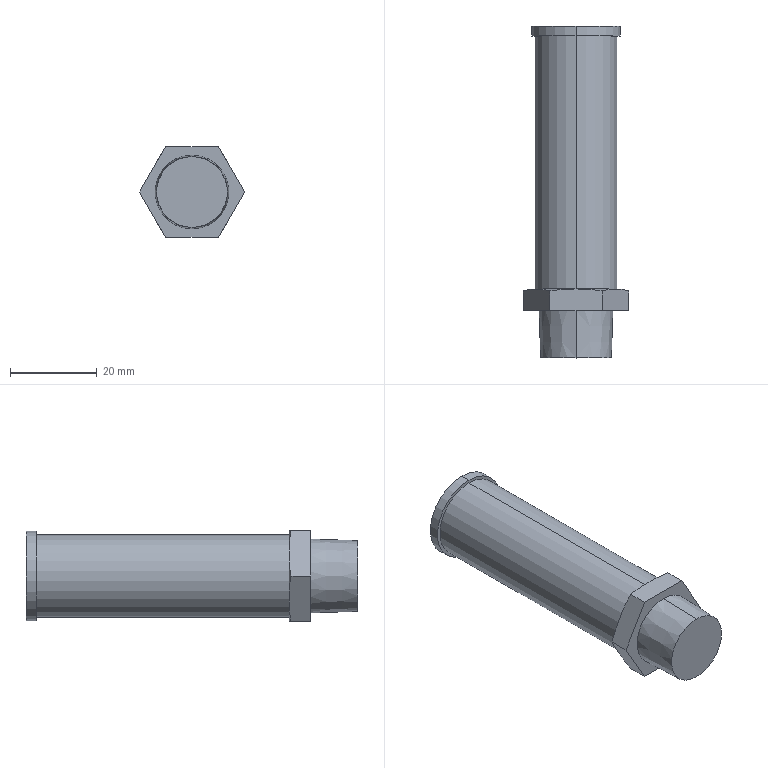Part | SolidWorks | features RefAxis 3, BaseBody 1, MoveFace 1 | 1 solid | 24 faces | box 24.249 x 76.6 x 21 mm | volume 21613 mm3 | plane 11 | cone 9 | cylinder 4 | commonest cylinder face diameters 19 x2 20.6 x2
STEP:
#1=CARTESIAN_POINT('',(0.,69.2,-9.5));
#2=VERTEX_POINT('',#1);
#3=CARTESIAN_POINT('',(0.,69.2,9.5));
#4=VERTEX_POINT('',#3);
#5=CARTESIAN_POINT('',(0.,69.2,0.));
#6=DIRECTION('',(0.,-1.,0.));
#7=DIRECTION('',(0.,0.,-1.));
#8=AXIS2_PLACEMENT_3D('',#5,#6,#7);
#9=CIRCLE('',#8,9.5);
#10=EDGE_CURVE('',#2,#4,#9,.T.);
#11=ORIENTED_EDGE('',*,*,#10,.T.);
#12=CARTESIAN_POINT('',(0.,10.8,9.5));
#13=VERTEX_POINT('',#12);
#14=CARTESIAN_POINT('',(0.,71.5,9.5));
#15=DIRECTION('',(0.,-1.,0.));
#16=VECTOR('',#15,1000.);
#17=LINE('',#14,#16);
#18=EDGE_CURVE('',#4,#13,#17,.T.);
#19=ORIENTED_EDGE('',*,*,#18,.T.);
#20=CARTESIAN_POINT('',(0.,10.8,-9.5));
#21=VERTEX_POINT('',#20);
#22=CARTESIAN_POINT('',(0.,10.8,0.));
#23=DIRECTION('',(0.,1.,0.));
#24=DIRECTION('',(0.,0.,-1.));
#25=AXIS2_PLACEMENT_3D('',#22,#23,#24);
#26=CIRCLE('',#25,9.5);
#27=EDGE_CURVE('',#13,#21,#26,.T.);
#28=ORIENTED_EDGE('',*,*,#27,.T.);
#29=CARTESIAN_POINT('',(0.,71.5,-9.5));
#30=DIRECTION('',(0.,-1.,0.));
#31=VECTOR('',#30,1000.);
#32=LINE('',#29,#31);
#33=EDGE_CURVE('',#2,#21,#32,.T.);
#34=ORIENTED_EDGE('',*,*,#33,.F.);
#35=EDGE_LOOP('',(#11,#19,#28,#34));
#36=FACE_OUTER_BOUND('',#35,.T.);
#37=CARTESIAN_POINT('',(0.,71.5,0.));
#38=DIRECTION('',(0.,-1.,0.));
#39=DIRECTION('',(0.,0.,-1.));
#40=AXIS2_PLACEMENT_3D('',#37,#38,#39);
#41=CYLINDRICAL_SURFACE('',#40,9.5);
#42=ADVANCED_FACE('',(#36),#41,.T.);
#43=CARTESIAN_POINT('',(9.093,10.8,-5.25));
#44=VERTEX_POINT('',#43);
#45=CARTESIAN_POINT('',(10.5,10.8,0.));
#46=VERTEX_POINT('',#45);
#47=CARTESIAN_POINT('',(0.,10.8,0.));
#48=DIRECTION('',(0.,-1.,0.));
#49=DIRECTION('',(1.,0.,0.));
#50=AXIS2_PLACEMENT_3D('',#47,#48,#49);
#51=CIRCLE('',#50,10.5);
#52=EDGE_CURVE('',#44,#46,#51,.T.);
#53=ORIENTED_EDGE('',*,*,#52,.T.);
#54=CARTESIAN_POINT('',(12.124,10.365,-0.000000011));
#55=VERTEX_POINT('',#54);
#56=CARTESIAN_POINT('',(12.134,10.362,0.));
#57=DIRECTION('',(0.9659,-0.2588,0.));
#58=VECTOR('',#57,1000.);
#59=LINE('',#56,#58);
#60=EDGE_CURVE('',#46,#55,#59,.T.);
#61=ORIENTED_EDGE('',*,*,#60,.T.);
#62=CARTESIAN_POINT('',(12.124,10.365,-0.000000011));
#63=CARTESIAN_POINT('',(11.621,10.5,-0.8711));
#64=CARTESIAN_POINT('',(11.118,10.609,-1.744));
#65=CARTESIAN_POINT('',(10.107,10.76,-3.493));
#66=CARTESIAN_POINT('',(9.601,10.8,-4.37));
#67=CARTESIAN_POINT('',(9.093,10.8,-5.25));
#68=B_SPLINE_CURVE_WITH_KNOTS('',3,(#62,#63,#64,#65,#66,#67),.UNSPECIFIED.,.F.,.F.,(4,2,4),(0.,0.003039,0.006078),.UNSPECIFIED.);
#69=EDGE_CURVE('',#55,#44,#68,.T.);
#70=ORIENTED_EDGE('',*,*,#69,.T.);
#71=EDGE_LOOP('',(#53,#61,#70));
#72=FACE_OUTER_BOUND('',#71,.T.);
#73=CARTESIAN_POINT('',(0.,10.362,0.));
#74=DIRECTION('',(0.,-1.,0.));
#75=DIRECTION('',(1.,0.,0.));
#76=AXIS2_PLACEMENT_3D('',#73,#74,#75);
#77=CONICAL_SURFACE('',#76,12.134,1.309);
#78=ADVANCED_FACE('',(#72),#77,.T.);
#79=CARTESIAN_POINT('',(0.,71.5,-10.3));
#80=VERTEX_POINT('',#79);
#81=CARTESIAN_POINT('',(0.,71.5,10.3));
#82=VERTEX_POINT('',#81);
#83=CARTESIAN_POINT('',(0.,71.5,0.));
#84=DIRECTION('',(0.,-1.,0.));
#85=DIRECTION('',(0.,0.,-1.));
#86=AXIS2_PLACEMENT_3D('',#83,#84,#85);
#87=CIRCLE('',#86,10.3);
#88=EDGE_CURVE('',#80,#82,#87,.T.);
#89=ORIENTED_EDGE('',*,*,#88,.T.);
#90=CARTESIAN_POINT('',(0.,69.2,10.3));
#91=VERTEX_POINT('',#90);
#92=CARTESIAN_POINT('',(0.,71.5,10.3));
#93=DIRECTION('',(0.,-1.,0.));
#94=VECTOR('',#93,1000.);
#95=LINE('',#92,#94);
#96=EDGE_CURVE('',#82,#91,#95,.T.);
#97=ORIENTED_EDGE('',*,*,#96,.T.);
#98=CARTESIAN_POINT('',(0.,69.2,-10.3));
#99=VERTEX_POINT('',#98);
#100=CARTESIAN_POINT('',(0.,69.2,0.));
#101=DIRECTION('',(0.,1.,0.));
#102=DIRECTION('',(0.,0.,-1.));
#103=AXIS2_PLACEMENT_3D('',#100,#101,#102);
#104=CIRCLE('',#103,10.3);
#105=EDGE_CURVE('',#91,#99,#104,.T.);
#106=ORIENTED_EDGE('',*,*,#105,.T.);
#107=CARTESIAN_POINT('',(0.,71.5,-10.3));
#108=DIRECTION('',(0.,-1.,0.));
#109=VECTOR('',#108,1000.);
#110=LINE('',#107,#109);
#111=EDGE_CURVE('',#80,#99,#110,.T.);
#112=ORIENTED_EDGE('',*,*,#111,.F.);
#113=EDGE_LOOP('',(#89,#97,#106,#112));
#114=FACE_OUTER_BOUND('',#113,.T.);
#115=CARTESIAN_POINT('',(0.,71.5,0.));
#116=DIRECTION('',(0.,-1.,0.));
#117=DIRECTION('',(0.,0.,-1.));
#118=AXIS2_PLACEMENT_3D('',#115,#116,#117);
#119=CYLINDRICAL_SURFACE('',#118,10.3);
#120=ADVANCED_FACE('',(#114),#119,.T.);
#121=CARTESIAN_POINT('',(0.,-5.1,8.172));
#122=VERTEX_POINT('',#121);
#123=CARTESIAN_POINT('',(0.,-5.1,-8.172));
#124=VERTEX_POINT('',#123);
#125=CARTESIAN_POINT('',(0.,-5.1,0.));
#126=DIRECTION('',(0.,1.,0.));
#127=DIRECTION('',(0.,0.,1.));
#128=AXIS2_PLACEMENT_3D('',#125,#126,#127);
#129=CIRCLE('',#128,8.172);
#130=EDGE_CURVE('',#122,#124,#129,.T.);
#131=ORIENTED_EDGE('',*,*,#130,.T.);
#132=CARTESIAN_POINT('',(0.,5.8,-8.512));
#133=VERTEX_POINT('',#132);
#134=CARTESIAN_POINT('',(0.,5.8,-8.512));
#135=DIRECTION('',(0.,0.9995,-0.0312));
#136=VECTOR('',#135,1000.);
#137=LINE('',#134,#136);
#138=EDGE_CURVE('',#124,#133,#137,.T.);
#139=ORIENTED_EDGE('',*,*,#138,.T.);
#140=CARTESIAN_POINT('',(0.,5.8,8.512));
#141=VERTEX_POINT('',#140);
#142=CARTESIAN_POINT('',(0.,5.8,0.));
#143=DIRECTION('',(0.,-1.,0.));
#144=DIRECTION('',(0.,0.,1.));
#145=AXIS2_PLACEMENT_3D('',#142,#143,#144);
#146=CIRCLE('',#145,8.512);
#147=EDGE_CURVE('',#133,#141,#146,.T.);
#148=ORIENTED_EDGE('',*,*,#147,.T.);
#149=CARTESIAN_POINT('',(0.,5.8,8.512));
#150=DIRECTION('',(0.,0.9995,0.0312));
#151=VECTOR('',#150,1000.);
#152=LINE('',#149,#151);
#153=EDGE_CURVE('',#122,#141,#152,.T.);
#154=ORIENTED_EDGE('',*,*,#153,.F.);
#155=EDGE_LOOP('',(#131,#139,#148,#154));
#156=FACE_OUTER_BOUND('',#155,.T.);
#157=CARTESIAN_POINT('',(0.,5.8,0.));
#158=DIRECTION('',(0.,1.,0.));
#159=DIRECTION('',(0.,0.,1.));
#160=AXIS2_PLACEMENT_3D('',#157,#158,#159);
#161=CONICAL_SURFACE('',#160,8.512,0.03121);
#162=ADVANCED_FACE('',(#156),#161,.T.);
#163=ORIENTED_EDGE('',*,*,#18,.F.);
#164=CARTESIAN_POINT('',(0.,69.2,0.));
#165=DIRECTION('',(0.,-1.,0.));
#166=DIRECTION('',(0.,0.,-1.));
#167=AXIS2_PLACEMENT_3D('',#164,#165,#166);
#168=CIRCLE('',#167,9.5);
#169=EDGE_CURVE('',#4,#2,#168,.T.);
#170=ORIENTED_EDGE('',*,*,#169,.T.);
#171=ORIENTED_EDGE('',*,*,#33,.T.);
#172=CARTESIAN_POINT('',(0.,10.8,0.));
#173=DIRECTION('',(0.,1.,0.));
#174=DIRECTION('',(0.,0.,-1.));
#175=AXIS2_PLACEMENT_3D('',#172,#173,#174);
#176=CIRCLE('',#175,9.5);
#177=EDGE_CURVE('',#21,#13,#176,.T.);
#178=ORIENTED_EDGE('',*,*,#177,.T.);
#179=EDGE_LOOP('',(#163,#170,#171,#178));
#180=FACE_OUTER_BOUND('',#179,.T.);
#181=CARTESIAN_POINT('',(0.,71.5,0.));
#182=DIRECTION('',(0.,-1.,0.));
#183=DIRECTION('',(0.,0.,-1.));
#184=AXIS2_PLACEMENT_3D('',#181,#182,#183);
#185=CYLINDRICAL_SURFACE('',#184,9.5);
#186=ADVANCED_FACE('',(#180),#185,.T.);
#187=CARTESIAN_POINT('',(-9.093,10.8,5.25));
#188=VERTEX_POINT('',#187);
#189=CARTESIAN_POINT('',(-9.093,10.8,-5.25));
#190=VERTEX_POINT('',#189);
#191=CARTESIAN_POINT('',(0.,10.8,0.));
#192=DIRECTION('',(0.,-1.,0.));
#193=DIRECTION('',(1.,0.,0.));
#194=AXIS2_PLACEMENT_3D('',#191,#192,#193);
#195=CIRCLE('',#194,10.5);
#196=EDGE_CURVE('',#188,#190,#195,.T.);
#197=ORIENTED_EDGE('',*,*,#196,.F.);
#198=CARTESIAN_POINT('',(0.,10.8,10.5));
#199=VERTEX_POINT('',#198);
#200=CARTESIAN_POINT('',(0.,10.8,0.));
#201=DIRECTION('',(0.,-1.,0.));
#202=DIRECTION('',(1.,0.,0.));
#203=AXIS2_PLACEMENT_3D('',#200,#201,#202);
#204=CIRCLE('',#203,10.5);
#205=EDGE_CURVE('',#199,#188,#204,.T.);
#206=ORIENTED_EDGE('',*,*,#205,.F.);
#207=CARTESIAN_POINT('',(9.093,10.8,5.25));
#208=VERTEX_POINT('',#207);
#209=CARTESIAN_POINT('',(0.,10.8,0.));
#210=DIRECTION('',(0.,-1.,0.));
#211=DIRECTION('',(1.,0.,0.));
#212=AXIS2_PLACEMENT_3D('',#209,#210,#211);
#213=CIRCLE('',#212,10.5);
#214=EDGE_CURVE('',#208,#199,#213,.T.);
#215=ORIENTED_EDGE('',*,*,#214,.F.);
#216=CARTESIAN_POINT('',(0.,10.8,0.));
#217=DIRECTION('',(0.,-1.,0.));
#218=DIRECTION('',(1.,0.,0.));
#219=AXIS2_PLACEMENT_3D('',#216,#217,#218);
#220=CIRCLE('',#219,10.5);
#221=EDGE_CURVE('',#46,#208,#220,.T.);
#222=ORIENTED_EDGE('',*,*,#221,.F.);
#223=ORIENTED_EDGE('',*,*,#52,.F.);
#224=CARTESIAN_POINT('',(0.,10.8,-10.5));
#225=VERTEX_POINT('',#224);
#226=CARTESIAN_POINT('',(0.,10.8,0.));
#227=DIRECTION('',(0.,-1.,0.));
#228=DIRECTION('',(1.,0.,0.));
#229=AXIS2_PLACEMENT_3D('',#226,#227,#228);
#230=CIRCLE('',#229,10.5);
#231=EDGE_CURVE('',#225,#44,#230,.T.);
#232=ORIENTED_EDGE('',*,*,#231,.F.);
#233=CARTESIAN_POINT('',(0.,10.8,0.));
#234=DIRECTION('',(0.,-1.,0.));
#235=DIRECTION('',(1.,0.,0.));
#236=AXIS2_PLACEMENT_3D('',#233,#234,#235);
#237=CIRCLE('',#236,10.5);
#238=EDGE_CURVE('',#190,#225,#237,.T.);
#239=ORIENTED_EDGE('',*,*,#238,.F.);
#240=EDGE_LOOP('',(#197,#206,#215,#222,#223,#232,#239));
#241=FACE_OUTER_BOUND('',#240,.T.);
#242=ORIENTED_EDGE('',*,*,#177,.F.);
#243=ORIENTED_EDGE('',*,*,#27,.F.);
#244=EDGE_LOOP('',(#242,#243));
#245=FACE_BOUND('',#244,.T.);
#246=CARTESIAN_POINT('',(-10.5,10.8,0.));
#247=DIRECTION('',(0.,-1.,0.));
#248=DIRECTION('',(0.,0.,-1.));
#249=AXIS2_PLACEMENT_3D('',#246,#247,#248);
#250=PLANE('',#249);
#251=ADVANCED_FACE('',(#241,#245),#250,.F.);
#252=ORIENTED_EDGE('',*,*,#10,.F.);
#253=ORIENTED_EDGE('',*,*,#169,.F.);
#254=EDGE_LOOP('',(#252,#253));
#255=FACE_BOUND('',#254,.T.);
#256=CARTESIAN_POINT('',(0.,69.2,0.));
#257=DIRECTION('',(0.,1.,0.));
#258=DIRECTION('',(0.,0.,-1.));
#259=AXIS2_PLACEMENT_3D('',#256,#257,#258);
#260=CIRCLE('',#259,10.3);
#261=EDGE_CURVE('',#99,#91,#260,.T.);
#262=ORIENTED_EDGE('',*,*,#261,.F.);
#263=ORIENTED_EDGE('',*,*,#105,.F.);
#264=EDGE_LOOP('',(#262,#263));
#265=FACE_OUTER_BOUND('',#264,.T.);
#266=CARTESIAN_POINT('',(-9.5,69.2,0.));
#267=DIRECTION('',(0.,1.,0.));
#268=DIRECTION('',(0.,0.,1.));
#269=AXIS2_PLACEMENT_3D('',#266,#267,#268);
#270=PLANE('',#269);
#271=ADVANCED_FACE('',(#255,#265),#270,.F.);
#272=CARTESIAN_POINT('',(-6.062,10.365,-10.5));
#273=VERTEX_POINT('',#272);
#274=CARTESIAN_POINT('',(0.,10.8,-10.5));
#275=CARTESIAN_POINT('',(-1.016,10.8,-10.5));
#276=CARTESIAN_POINT('',(-2.028,10.76,-10.5));
#277=CARTESIAN_POINT('',(-4.049,10.609,-10.5));
#278=CARTESIAN_POINT('',(-5.056,10.5,-10.5));
#279=CARTESIAN_POINT('',(-6.062,10.365,-10.5));
#280=B_SPLINE_CURVE_WITH_KNOTS('',3,(#274,#275,#276,#277,#278,#279),.UNSPECIFIED.,.F.,.F.,(4,2,4),(0.,0.003039,0.006078),.UNSPECIFIED.);
#281=EDGE_CURVE('',#225,#273,#280,.T.);
#282=ORIENTED_EDGE('',*,*,#281,.T.);
#283=CARTESIAN_POINT('',(-6.062,10.365,-10.5));
#284=CARTESIAN_POINT('',(-6.565,10.5,-9.629));
#285=CARTESIAN_POINT('',(-7.069,10.609,-8.756));
#286=CARTESIAN_POINT('',(-8.079,10.76,-7.007));
#287=CARTESIAN_POINT('',(-8.585,10.8,-6.13));
#288=CARTESIAN_POINT('',(-9.093,10.8,-5.25));
#289=B_SPLINE_CURVE_WITH_KNOTS('',3,(#283,#284,#285,#286,#287,#288),.UNSPECIFIED.,.F.,.F.,(4,2,4),(0.,0.003039,0.006078),.UNSPECIFIED.);
#290=EDGE_CURVE('',#273,#190,#289,.T.);
#291=ORIENTED_EDGE('',*,*,#290,.T.);
#292=ORIENTED_EDGE('',*,*,#238,.T.);
#293=EDGE_LOOP('',(#282,#291,#292));
#294=FACE_OUTER_BOUND('',#293,.T.);
#295=CARTESIAN_POINT('',(0.,10.362,0.));
#296=DIRECTION('',(0.,-1.,0.));
#297=DIRECTION('',(1.,0.,0.));
#298=AXIS2_PLACEMENT_3D('',#295,#296,#297);
#299=CONICAL_SURFACE('',#298,12.134,1.309);
#300=ADVANCED_FACE('',(#294),#299,.T.);
#301=CARTESIAN_POINT('',(-12.124,10.365,-0.00000002));
#302=VERTEX_POINT('',#301);
#303=CARTESIAN_POINT('',(-9.093,10.8,-5.25));
#304=CARTESIAN_POINT('',(-9.601,10.8,-4.37));
#305=CARTESIAN_POINT('',(-10.107,10.76,-3.493));
#306=CARTESIAN_POINT('',(-11.118,10.609,-1.744));
#307=CARTESIAN_POINT('',(-11.621,10.5,-0.8711));
#308=CARTESIAN_POINT('',(-12.124,10.365,-0.00000002));
#309=B_SPLINE_CURVE_WITH_KNOTS('',3,(#303,#304,#305,#306,#307,#308),.UNSPECIFIED.,.F.,.F.,(4,2,4),(0.,0.003039,0.006078),.UNSPECIFIED.);
#310=EDGE_CURVE('',#190,#302,#309,.T.);
#311=ORIENTED_EDGE('',*,*,#310,.T.);
#312=CARTESIAN_POINT('',(-12.124,10.365,-0.00000002));
#313=CARTESIAN_POINT('',(-11.621,10.5,0.8711));
#314=CARTESIAN_POINT('',(-11.118,10.609,1.744));
#315=CARTESIAN_POINT('',(-10.107,10.76,3.493));
#316=CARTESIAN_POINT('',(-9.601,10.8,4.37));
#317=CARTESIAN_POINT('',(-9.093,10.8,5.25));
#318=B_SPLINE_CURVE_WITH_KNOTS('',3,(#312,#313,#314,#315,#316,#317),.UNSPECIFIED.,.F.,.F.,(4,2,4),(0.,0.003039,0.006078),.UNSPECIFIED.);
#319=EDGE_CURVE('',#302,#188,#318,.T.);
#320=ORIENTED_EDGE('',*,*,#319,.T.);
#321=ORIENTED_EDGE('',*,*,#196,.T.);
#322=EDGE_LOOP('',(#311,#320,#321));
#323=FACE_OUTER_BOUND('',#322,.T.);
#324=CARTESIAN_POINT('',(0.,10.362,0.));
#325=DIRECTION('',(0.,-1.,0.));
#326=DIRECTION('',(1.,0.,0.));
#327=AXIS2_PLACEMENT_3D('',#324,#325,#326);
#328=CONICAL_SURFACE('',#327,12.134,1.309);
#329=ADVANCED_FACE('',(#323),#328,.T.);
#330=CARTESIAN_POINT('',(-6.062,10.365,10.5));
#331=VERTEX_POINT('',#330);
#332=CARTESIAN_POINT('',(-6.062,10.365,10.5));
#333=CARTESIAN_POINT('',(-5.056,10.5,10.5));
#334=CARTESIAN_POINT('',(-4.049,10.609,10.5));
#335=CARTESIAN_POINT('',(-2.028,10.76,10.5));
#336=CARTESIAN_POINT('',(-1.016,10.8,10.5));
#337=CARTESIAN_POINT('',(0.,10.8,10.5));
#338=B_SPLINE_CURVE_WITH_KNOTS('',3,(#332,#333,#334,#335,#336,#337),.UNSPECIFIED.,.F.,.F.,(4,2,4),(0.,0.003039,0.006078),.UNSPECIFIED.);
#339=EDGE_CURVE('',#331,#199,#338,.T.);
#340=ORIENTED_EDGE('',*,*,#339,.T.);
#341=ORIENTED_EDGE('',*,*,#205,.T.);
#342=CARTESIAN_POINT('',(-9.093,10.8,5.25));
#343=CARTESIAN_POINT('',(-8.585,10.8,6.13));
#344=CARTESIAN_POINT('',(-8.079,10.76,7.007));
#345=CARTESIAN_POINT('',(-7.069,10.609,8.756));
#346=CARTESIAN_POINT('',(-6.565,10.5,9.629));
#347=CARTESIAN_POINT('',(-6.062,10.365,10.5));
#348=B_SPLINE_CURVE_WITH_KNOTS('',3,(#342,#343,#344,#345,#346,#347),.UNSPECIFIED.,.F.,.F.,(4,2,4),(0.,0.003039,0.006078),.UNSPECIFIED.);
#349=EDGE_CURVE('',#188,#331,#348,.T.);
#350=ORIENTED_EDGE('',*,*,#349,.T.);
#351=EDGE_LOOP('',(#340,#341,#350));
#352=FACE_OUTER_BOUND('',#351,.T.);
#353=CARTESIAN_POINT('',(0.,10.362,0.));
#354=DIRECTION('',(0.,-1.,0.));
#355=DIRECTION('',(1.,0.,0.));
#356=AXIS2_PLACEMENT_3D('',#353,#354,#355);
#357=CONICAL_SURFACE('',#356,12.134,1.309);
#358=ADVANCED_FACE('',(#352),#357,.T.);
#359=CARTESIAN_POINT('',(6.062,10.365,10.5));
#360=VERTEX_POINT('',#359);
#361=CARTESIAN_POINT('',(6.062,10.365,10.5));
#362=CARTESIAN_POINT('',(6.565,10.5,9.629));
#363=CARTESIAN_POINT('',(7.069,10.609,8.756));
#364=CARTESIAN_POINT('',(8.079,10.76,7.007));
#365=CARTESIAN_POINT('',(8.585,10.8,6.13));
#366=CARTESIAN_POINT('',(9.093,10.8,5.25));
#367=B_SPLINE_CURVE_WITH_KNOTS('',3,(#361,#362,#363,#364,#365,#366),.UNSPECIFIED.,.F.,.F.,(4,2,4),(0.,0.003039,0.006078),.UNSPECIFIED.);
#368=EDGE_CURVE('',#360,#208,#367,.T.);
#369=ORIENTED_EDGE('',*,*,#368,.T.);
#370=ORIENTED_EDGE('',*,*,#214,.T.);
#371=CARTESIAN_POINT('',(0.,10.8,10.5));
#372=CARTESIAN_POINT('',(1.016,10.8,10.5));
#373=CARTESIAN_POINT('',(2.028,10.76,10.5));
#374=CARTESIAN_POINT('',(4.049,10.609,10.5));
#375=CARTESIAN_POINT('',(5.056,10.5,10.5));
#376=CARTESIAN_POINT('',(6.062,10.365,10.5));
#377=B_SPLINE_CURVE_WITH_KNOTS('',3,(#371,#372,#373,#374,#375,#376),.UNSPECIFIED.,.F.,.F.,(4,2,4),(0.,0.003039,0.006078),.UNSPECIFIED.);
#378=EDGE_CURVE('',#199,#360,#377,.T.);
#379=ORIENTED_EDGE('',*,*,#378,.T.);
#380=EDGE_LOOP('',(#369,#370,#379));
#381=FACE_OUTER_BOUND('',#380,.T.);
#382=CARTESIAN_POINT('',(0.,10.362,0.));
#383=DIRECTION('',(0.,-1.,0.));
#384=DIRECTION('',(1.,0.,0.));
#385=AXIS2_PLACEMENT_3D('',#382,#383,#384);
#386=CONICAL_SURFACE('',#385,12.134,1.309);
#387=ADVANCED_FACE('',(#381),#386,.T.);
#388=ORIENTED_EDGE('',*,*,#60,.F.);
#389=ORIENTED_EDGE('',*,*,#221,.T.);
#390=CARTESIAN_POINT('',(9.093,10.8,5.25));
#391=CARTESIAN_POINT('',(9.601,10.8,4.37));
#392=CARTESIAN_POINT('',(10.107,10.76,3.493));
#393=CARTESIAN_POINT('',(11.118,10.609,1.744));
#394=CARTESIAN_POINT('',(11.621,10.5,0.8711));
#395=CARTESIAN_POINT('',(12.124,10.365,-0.000000011));
#396=B_SPLINE_CURVE_WITH_KNOTS('',3,(#390,#391,#392,#393,#394,#395),.UNSPECIFIED.,.F.,.F.,(4,2,4),(0.,0.003039,0.006078),.UNSPECIFIED.);
#397=EDGE_CURVE('',#208,#55,#396,.T.);
#398=ORIENTED_EDGE('',*,*,#397,.T.);
#399=EDGE_LOOP('',(#388,#389,#398));
#400=FACE_OUTER_BOUND('',#399,.T.);
#401=CARTESIAN_POINT('',(0.,10.362,0.));
#402=DIRECTION('',(0.,-1.,0.));
#403=DIRECTION('',(1.,0.,0.));
#404=AXIS2_PLACEMENT_3D('',#401,#402,#403);
#405=CONICAL_SURFACE('',#404,12.134,1.309);
#406=ADVANCED_FACE('',(#400),#405,.T.);
#407=CARTESIAN_POINT('',(6.062,10.365,-10.5));
#408=VERTEX_POINT('',#407);
#409=CARTESIAN_POINT('',(9.093,10.8,-5.25));
#410=CARTESIAN_POINT('',(8.585,10.8,-6.13));
#411=CARTESIAN_POINT('',(8.079,10.76,-7.007));
#412=CARTESIAN_POINT('',(7.069,10.609,-8.756));
#413=CARTESIAN_POINT('',(6.565,10.5,-9.629));
#414=CARTESIAN_POINT('',(6.062,10.365,-10.5));
#415=B_SPLINE_CURVE_WITH_KNOTS('',3,(#409,#410,#411,#412,#413,#414),.UNSPECIFIED.,.F.,.F.,(4,2,4),(0.,0.003039,0.006078),.UNSPECIFIED.);
#416=EDGE_CURVE('',#44,#408,#415,.T.);
#417=ORIENTED_EDGE('',*,*,#416,.T.);
#418=CARTESIAN_POINT('',(6.062,10.365,-10.5));
#419=CARTESIAN_POINT('',(5.056,10.5,-10.5));
#420=CARTESIAN_POINT('',(4.049,10.609,-10.5));
#421=CARTESIAN_POINT('',(2.028,10.76,-10.5));
#422=CARTESIAN_POINT('',(1.016,10.8,-10.5));
#423=CARTESIAN_POINT('',(0.,10.8,-10.5));
#424=B_SPLINE_CURVE_WITH_KNOTS('',3,(#418,#419,#420,#421,#422,#423),.UNSPECIFIED.,.F.,.F.,(4,2,4),(0.,0.003039,0.006078),.UNSPECIFIED.);
#425=EDGE_CURVE('',#408,#225,#424,.T.);
#426=ORIENTED_EDGE('',*,*,#425,.T.);
#427=ORIENTED_EDGE('',*,*,#231,.T.);
#428=EDGE_LOOP('',(#417,#426,#427));
#429=FACE_OUTER_BOUND('',#428,.T.);
#430=CARTESIAN_POINT('',(0.,10.362,0.));
#431=DIRECTION('',(0.,-1.,0.));
#432=DIRECTION('',(1.,0.,0.));
#433=AXIS2_PLACEMENT_3D('',#430,#431,#432);
#434=CONICAL_SURFACE('',#433,12.134,1.309);
#435=ADVANCED_FACE('',(#429),#434,.T.);
#436=ORIENTED_EDGE('',*,*,#96,.F.);
#437=CARTESIAN_POINT('',(0.,71.5,0.));
#438=DIRECTION('',(0.,-1.,0.));
#439=DIRECTION('',(0.,0.,-1.));
#440=AXIS2_PLACEMENT_3D('',#437,#438,#439);
#441=CIRCLE('',#440,10.3);
#442=EDGE_CURVE('',#82,#80,#441,.T.);
#443=ORIENTED_EDGE('',*,*,#442,.T.);
#444=ORIENTED_EDGE('',*,*,#111,.T.);
#445=ORIENTED_EDGE('',*,*,#261,.T.);
#446=EDGE_LOOP('',(#436,#443,#444,#445));
#447=FACE_OUTER_BOUND('',#446,.T.);
#448=CARTESIAN_POINT('',(0.,71.5,0.));
#449=DIRECTION('',(0.,-1.,0.));
#450=DIRECTION('',(0.,0.,-1.));
#451=AXIS2_PLACEMENT_3D('',#448,#449,#450);
#452=CYLINDRICAL_SURFACE('',#451,10.3);
#453=ADVANCED_FACE('',(#447),#452,.T.);
#454=ORIENTED_EDGE('',*,*,#310,.F.);
#455=ORIENTED_EDGE('',*,*,#290,.F.);
#456=CARTESIAN_POINT('',(-6.062,5.8,-10.5));
#457=VERTEX_POINT('',#456);
#458=CARTESIAN_POINT('',(-6.062,10.8,-10.5));
#459=DIRECTION('',(0.,1.,0.));
#460=VECTOR('',#459,1000.);
#461=LINE('',#458,#460);
#462=EDGE_CURVE('',#457,#273,#461,.T.);
#463=ORIENTED_EDGE('',*,*,#462,.F.);
#464=CARTESIAN_POINT('',(-12.124,5.8,0.));
#465=VERTEX_POINT('',#464);
#466=CARTESIAN_POINT('',(-6.062,5.8,-10.5));
#467=DIRECTION('',(0.5,0.,-0.866));
#468=VECTOR('',#467,1000.);
#469=LINE('',#466,#468);
#470=EDGE_CURVE('',#465,#457,#469,.T.);
#471=ORIENTED_EDGE('',*,*,#470,.F.);
#472=CARTESIAN_POINT('',(-12.124,10.8,0.));
#473=DIRECTION('',(0.,-1.,0.));
#474=VECTOR('',#473,1000.);
#475=LINE('',#472,#474);
#476=EDGE_CURVE('',#302,#465,#475,.T.);
#477=ORIENTED_EDGE('',*,*,#476,.F.);
#478=EDGE_LOOP('',(#454,#455,#463,#471,#477));
#479=FACE_OUTER_BOUND('',#478,.T.);
#480=CARTESIAN_POINT('',(-6.062,10.8,-10.5));
#481=DIRECTION('',(0.866,0.,0.5));
#482=DIRECTION('',(0.5,0.,-0.866));
#483=AXIS2_PLACEMENT_3D('',#480,#481,#482);
#484=PLANE('',#483);
#485=ADVANCED_FACE('',(#479),#484,.F.);
#486=ORIENTED_EDGE('',*,*,#281,.F.);
#487=ORIENTED_EDGE('',*,*,#425,.F.);
#488=CARTESIAN_POINT('',(6.062,5.8,-10.5));
#489=VERTEX_POINT('',#488);
#490=CARTESIAN_POINT('',(6.062,10.8,-10.5));
#491=DIRECTION('',(0.,1.,0.));
#492=VECTOR('',#491,1000.);
#493=LINE('',#490,#492);
#494=EDGE_CURVE('',#489,#408,#493,.T.);
#495=ORIENTED_EDGE('',*,*,#494,.F.);
#496=CARTESIAN_POINT('',(6.062,5.8,-10.5));
#497=DIRECTION('',(1.,0.,0.));
#498=VECTOR('',#497,1000.);
#499=LINE('',#496,#498);
#500=EDGE_CURVE('',#457,#489,#499,.T.);
#501=ORIENTED_EDGE('',*,*,#500,.F.);
#502=ORIENTED_EDGE('',*,*,#462,.T.);
#503=EDGE_LOOP('',(#486,#487,#495,#501,#502));
#504=FACE_OUTER_BOUND('',#503,.T.);
#505=CARTESIAN_POINT('',(6.062,10.8,-10.5));
#506=DIRECTION('',(0.,0.,1.));
#507=DIRECTION('',(1.,0.,0.));
#508=AXIS2_PLACEMENT_3D('',#505,#506,#507);
#509=PLANE('',#508);
#510=ADVANCED_FACE('',(#504),#509,.F.);
#511=ORIENTED_EDGE('',*,*,#349,.F.);
#512=ORIENTED_EDGE('',*,*,#319,.F.);
#513=ORIENTED_EDGE('',*,*,#476,.T.);
#514=CARTESIAN_POINT('',(-6.062,5.8,10.5));
#515=VERTEX_POINT('',#514);
#516=CARTESIAN_POINT('',(-12.124,5.8,0.));
#517=DIRECTION('',(-0.5,0.,-0.866));
#518=VECTOR('',#517,1000.);
#519=LINE('',#516,#518);
#520=EDGE_CURVE('',#515,#465,#519,.T.);
#521=ORIENTED_EDGE('',*,*,#520,.F.);
#522=CARTESIAN_POINT('',(-6.062,10.8,10.5));
#523=DIRECTION('',(0.,-1.,0.));
#524=VECTOR('',#523,1000.);
#525=LINE('',#522,#524);
#526=EDGE_CURVE('',#331,#515,#525,.T.);
#527=ORIENTED_EDGE('',*,*,#526,.F.);
#528=EDGE_LOOP('',(#511,#512,#513,#521,#527));
#529=FACE_OUTER_BOUND('',#528,.T.);
#530=CARTESIAN_POINT('',(-12.124,10.8,0.));
#531=DIRECTION('',(0.866,0.,-0.5));
#532=DIRECTION('',(-0.5,0.,-0.866));
#533=AXIS2_PLACEMENT_3D('',#530,#531,#532);
#534=PLANE('',#533);
#535=ADVANCED_FACE('',(#529),#534,.F.);
#536=ORIENTED_EDGE('',*,*,#378,.F.);
#537=ORIENTED_EDGE('',*,*,#339,.F.);
#538=ORIENTED_EDGE('',*,*,#526,.T.);
#539=CARTESIAN_POINT('',(6.062,5.8,10.5));
#540=VERTEX_POINT('',#539);
#541=CARTESIAN_POINT('',(-6.062,5.8,10.5));
#542=DIRECTION('',(-1.,0.,0.));
#543=VECTOR('',#542,1000.);
#544=LINE('',#541,#543);
#545=EDGE_CURVE('',#540,#515,#544,.T.);
#546=ORIENTED_EDGE('',*,*,#545,.F.);
#547=CARTESIAN_POINT('',(6.062,10.8,10.5));
#548=DIRECTION('',(0.,-1.,0.));
#549=VECTOR('',#548,1000.);
#550=LINE('',#547,#549);
#551=EDGE_CURVE('',#360,#540,#550,.T.);
#552=ORIENTED_EDGE('',*,*,#551,.F.);
#553=EDGE_LOOP('',(#536,#537,#538,#546,#552));
#554=FACE_OUTER_BOUND('',#553,.T.);
#555=CARTESIAN_POINT('',(-6.062,10.8,10.5));
#556=DIRECTION('',(0.,0.,-1.));
#557=DIRECTION('',(-1.,0.,0.));
#558=AXIS2_PLACEMENT_3D('',#555,#556,#557);
#559=PLANE('',#558);
#560=ADVANCED_FACE('',(#554),#559,.F.);
#561=ORIENTED_EDGE('',*,*,#397,.F.);
#562=ORIENTED_EDGE('',*,*,#368,.F.);
#563=ORIENTED_EDGE('',*,*,#551,.T.);
#564=CARTESIAN_POINT('',(12.124,5.8,0.));
#565=VERTEX_POINT('',#564);
#566=CARTESIAN_POINT('',(6.062,5.8,10.5));
#567=DIRECTION('',(-0.5,0.,0.866));
#568=VECTOR('',#567,1000.);
#569=LINE('',#566,#568);
#570=EDGE_CURVE('',#565,#540,#569,.T.);
#571=ORIENTED_EDGE('',*,*,#570,.F.);
#572=CARTESIAN_POINT('',(12.124,10.8,0.));
#573=DIRECTION('',(0.,-1.,0.));
#574=VECTOR('',#573,1000.);
#575=LINE('',#572,#574);
#576=EDGE_CURVE('',#55,#565,#575,.T.);
#577=ORIENTED_EDGE('',*,*,#576,.F.);
#578=EDGE_LOOP('',(#561,#562,#563,#571,#577));
#579=FACE_OUTER_BOUND('',#578,.T.);
#580=CARTESIAN_POINT('',(6.062,10.8,10.5));
#581=DIRECTION('',(-0.866,0.,-0.5));
#582=DIRECTION('',(-0.5,0.,0.866));
#583=AXIS2_PLACEMENT_3D('',#580,#581,#582);
#584=PLANE('',#583);
#585=ADVANCED_FACE('',(#579),#584,.F.);
#586=ORIENTED_EDGE('',*,*,#416,.F.);
#587=ORIENTED_EDGE('',*,*,#69,.F.);
#588=ORIENTED_EDGE('',*,*,#576,.T.);
#589=CARTESIAN_POINT('',(12.124,5.8,0.));
#590=DIRECTION('',(0.5,0.,0.866));
#591=VECTOR('',#590,1000.);
#592=LINE('',#589,#591);
#593=EDGE_CURVE('',#489,#565,#592,.T.);
#594=ORIENTED_EDGE('',*,*,#593,.F.);
#595=ORIENTED_EDGE('',*,*,#494,.T.);
#596=EDGE_LOOP('',(#586,#587,#588,#594,#595));
#597=FACE_OUTER_BOUND('',#596,.T.);
#598=CARTESIAN_POINT('',(12.124,10.8,0.));
#599=DIRECTION('',(-0.866,0.,0.5));
#600=DIRECTION('',(0.5,0.,0.866));
#601=AXIS2_PLACEMENT_3D('',#598,#599,#600);
#602=PLANE('',#601);
#603=ADVANCED_FACE('',(#597),#602,.F.);
#604=ORIENTED_EDGE('',*,*,#88,.F.);
#605=ORIENTED_EDGE('',*,*,#442,.F.);
#606=EDGE_LOOP('',(#604,#605));
#607=FACE_OUTER_BOUND('',#606,.T.);
#608=CARTESIAN_POINT('',(-10.3,71.5,0.));
#609=DIRECTION('',(0.,-1.,0.));
#610=DIRECTION('',(0.,0.,-1.));
#611=AXIS2_PLACEMENT_3D('',#608,#609,#610);
#612=PLANE('',#611);
#613=ADVANCED_FACE('',(#607),#612,.F.);
#614=CARTESIAN_POINT('',(0.,5.8,0.));
#615=DIRECTION('',(0.,-1.,0.));
#616=DIRECTION('',(0.,0.,1.));
#617=AXIS2_PLACEMENT_3D('',#614,#615,#616);
#618=CIRCLE('',#617,8.512);
#619=EDGE_CURVE('',#141,#133,#618,.T.);
#620=ORIENTED_EDGE('',*,*,#619,.F.);
#621=ORIENTED_EDGE('',*,*,#147,.F.);
#622=EDGE_LOOP('',(#620,#621));
#623=FACE_BOUND('',#622,.T.);
#624=ORIENTED_EDGE('',*,*,#470,.T.);
#625=ORIENTED_EDGE('',*,*,#500,.T.);
#626=ORIENTED_EDGE('',*,*,#593,.T.);
#627=ORIENTED_EDGE('',*,*,#570,.T.);
#628=ORIENTED_EDGE('',*,*,#545,.T.);
#629=ORIENTED_EDGE('',*,*,#520,.T.);
#630=EDGE_LOOP('',(#624,#625,#626,#627,#628,#629));
#631=FACE_OUTER_BOUND('',#630,.T.);
#632=CARTESIAN_POINT('',(-8.512,5.8,0.));
#633=DIRECTION('',(0.,1.,0.));
#634=DIRECTION('',(0.,0.,1.));
#635=AXIS2_PLACEMENT_3D('',#632,#633,#634);
#636=PLANE('',#635);
#637=ADVANCED_FACE('',(#623,#631),#636,.F.);
#638=ORIENTED_EDGE('',*,*,#138,.F.);
#639=CARTESIAN_POINT('',(0.,-5.1,0.));
#640=DIRECTION('',(0.,1.,0.));
#641=DIRECTION('',(0.,0.,1.));
#642=AXIS2_PLACEMENT_3D('',#639,#640,#641);
#643=CIRCLE('',#642,8.172);
#644=EDGE_CURVE('',#124,#122,#643,.T.);
#645=ORIENTED_EDGE('',*,*,#644,.T.);
#646=ORIENTED_EDGE('',*,*,#153,.T.);
#647=ORIENTED_EDGE('',*,*,#619,.T.);
#648=EDGE_LOOP('',(#638,#645,#646,#647));
#649=FACE_OUTER_BOUND('',#648,.T.);
#650=CARTESIAN_POINT('',(0.,5.8,0.));
#651=DIRECTION('',(0.,1.,0.));
#652=DIRECTION('',(0.,0.,1.));
#653=AXIS2_PLACEMENT_3D('',#650,#651,#652);
#654=CONICAL_SURFACE('',#653,8.512,0.03121);
#655=ADVANCED_FACE('',(#649),#654,.T.);
#656=ORIENTED_EDGE('',*,*,#130,.F.);
#657=ORIENTED_EDGE('',*,*,#644,.F.);
#658=EDGE_LOOP('',(#656,#657));
#659=FACE_OUTER_BOUND('',#658,.T.);
#660=CARTESIAN_POINT('',(10.5,-5.1,21.));
#661=DIRECTION('',(0.,-1.,0.));
#662=DIRECTION('',(0.,0.,-1.));
#663=AXIS2_PLACEMENT_3D('',#660,#661,#662);
#664=PLANE('',#663);
#665=ADVANCED_FACE('',(#659),#664,.T.);
#666=CLOSED_SHELL('',(#42,#78,#120,#162,#186,#251,#271,#300,#329,#358,#387,#406,#435,#453,#485,#510,#535,#560,#585,#603,#613,#637,#655,#665));
#667=MANIFOLD_SOLID_BREP('',#666);
#668=CARTESIAN_POINT('',(0.,0.,0.));
#669=DIRECTION('',(0.,0.,1.));
#670=DIRECTION('',(1.,0.,0.));
#671=AXIS2_PLACEMENT_3D('',#668,#669,#670);
#672=(LENGTH_UNIT()NAMED_UNIT(*)SI_UNIT(.MILLI.,.METRE.));
#673=UNCERTAINTY_MEASURE_WITH_UNIT(LENGTH_MEASURE(0.00001),#672,'','');
#674=(NAMED_UNIT(*)PLANE_ANGLE_UNIT()SI_UNIT($,.RADIAN.));
#675=(NAMED_UNIT(*)SI_UNIT($,.STERADIAN.)SOLID_ANGLE_UNIT());
#676=(GEOMETRIC_REPRESENTATION_CONTEXT(3)GLOBAL_UNCERTAINTY_ASSIGNED_CONTEXT((#673))GLOBAL_UNIT_ASSIGNED_CONTEXT((#672,#674,#675))REPRESENTATION_CONTEXT('',''));
#677=ADVANCED_BREP_SHAPE_REPRESENTATION('',(#667,#671),#676);